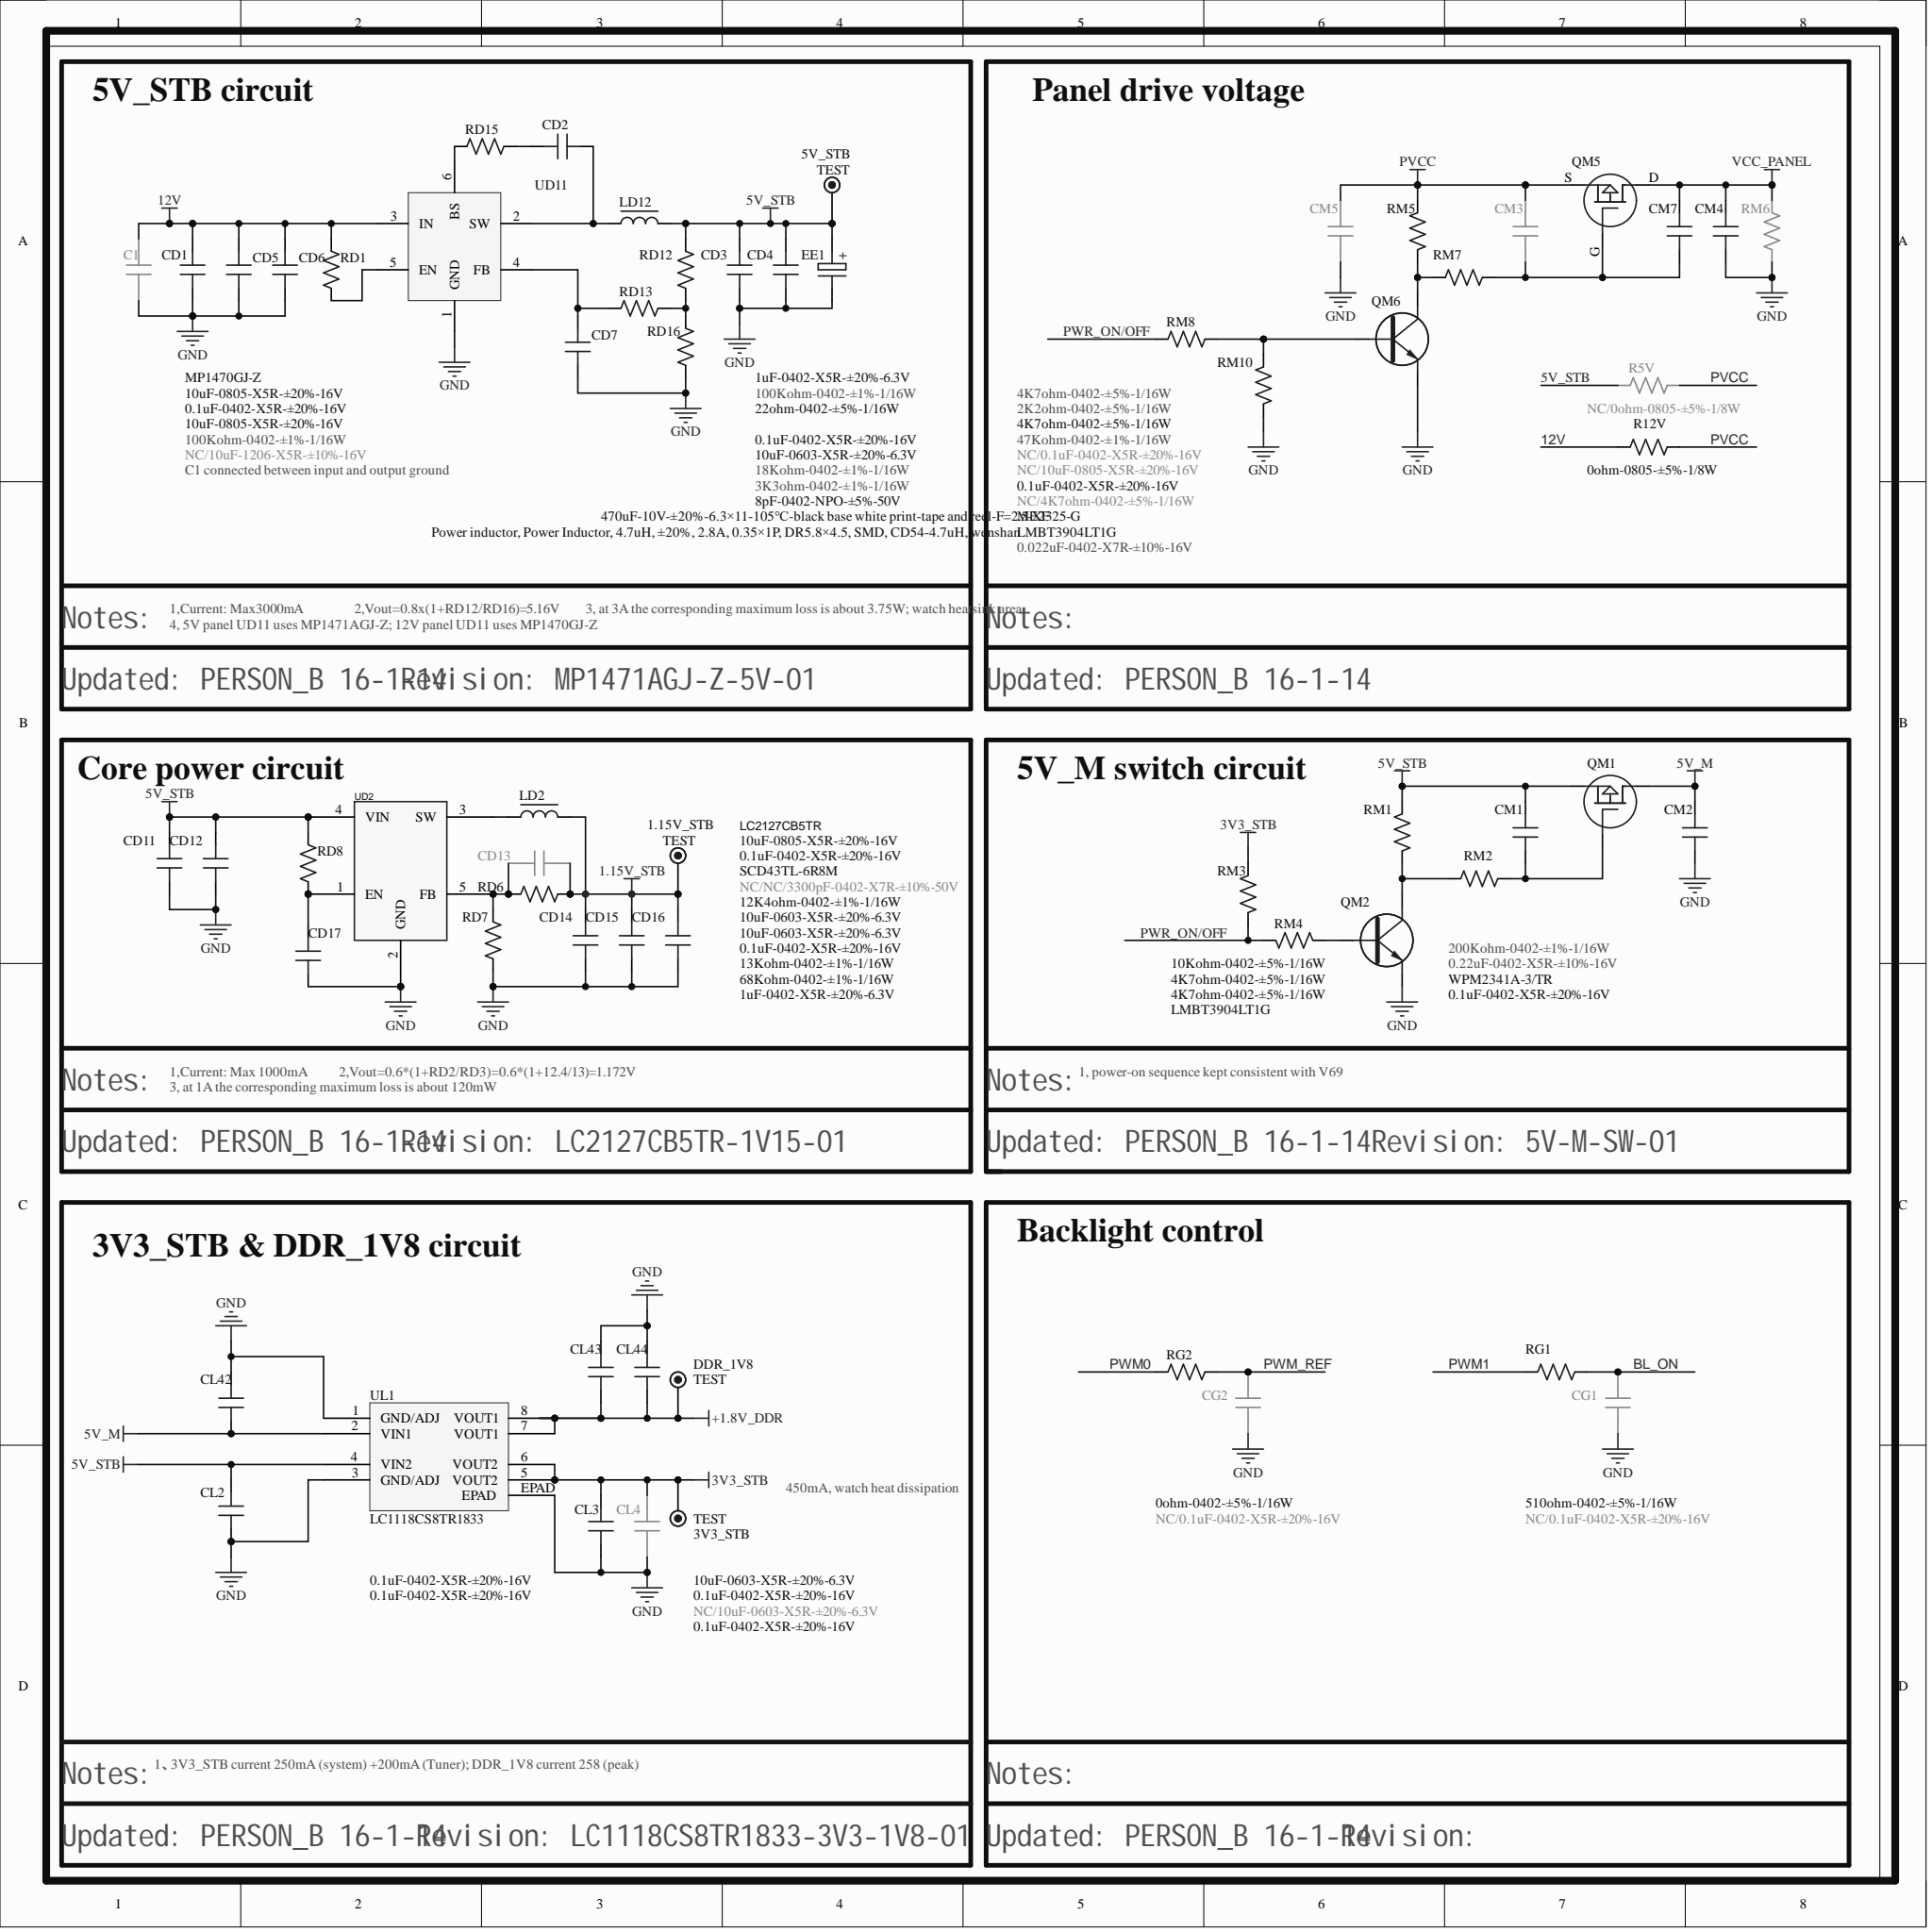Circuit board | Altium Designer | 709 parts | 378 nets | one sheet of the schematic
Parts on this sheet (reference | value | footprint):
1.15V_STB | TEST | TP
3V3_STB | TEST | TP
5V_STB | TEST | TP
BL_ON | TEST | TP_BL
C1 | NC/10uF-1206-X5R-±10%-16V | C1206
CD1 | 10uF-0805-X5R-±20%-16V | C0805
CD2 | 1uF-0402-X5R-±20%-6.3V | C0402
CD3 | 0.1uF-0402-X5R-±20%-16V | C0402
CD4 | 10uF-0603-X5R-±20%-6.3V | C0603
CD5 | 10uF-0805-X5R-±20%-16V | C0805
CD6 | 0.1uF-0402-X5R-±20%-16V | C0402
CD7 | 8pF-0402-NPO-±5%-50V | C0402
CD11 | 10uF-0805-X5R-±20%-16V | C0805
CD12 | 0.1uF-0402-X5R-±20%-16V | C0402
CD13 | NC/NC/3300pF-0402-X7R-±10%-50V | C0402
CD14 | 10uF-0603-X5R-±20%-6.3V | C0603
CD15 | 10uF-0603-X5R-±20%-6.3V | C0603
CD16 | 0.1uF-0402-X5R-±20%-16V | C0402
CD17 | 1uF-0402-X5R-±20%-6.3V | C0402
CG1 | NC/0.1uF-0402-X5R-±20%-16V | C0402
CG2 | NC/0.1uF-0402-X5R-±20%-16V | C0402
CL2 | 0.1uF-0402-X5R-±20%-16V | C0402
CL3 | 0.1uF-0402-X5R-±20%-16V | C0402
CL4 | NC/10uF-0603-X5R-±20%-6.3V | C0603
CL42 | 0.1uF-0402-X5R-±20%-16V | C0402
CL43 | 0.1uF-0402-X5R-±20%-16V | C0402
CL44 | 10uF-0603-X5R-±20%-6.3V | C0603
CM1 | 0.22uF-0402-X5R-±10%-16V | C0402
CM2 | 0.1uF-0402-X5R-±20%-16V | C0402
CM3 | NC/0.1uF-0402-X5R-±20%-16V | C0402
CM4 | 0.1uF-0402-X5R-±20%-16V | C0402
CM5 | NC/10uF-0805-X5R-±20%-16V | C0805
CM7 | 0.022uF-0402-X7R-±10%-16V | C0402
DDR_1V8 | TEST | TP
EE1 | 470uF-10V-±20%-6.3×11-105℃-black base white print-tape and reel-F=2.5-XF | EC(6.3*11)-V-2.5
LD2 | SCD43TL-6R8M | L(4.5*3.5)-S
LD12 | Power inductor, Power Inductor, 4.7uH, ±20%, 2.8A, 0.35×1P, DR5.8×4.5, SMD, CD54-4.7uH, wenshan | L(5.8*4.5)-S
PWM_REF | TEST | TP_BL
QM1 | WPM2341A-3/TR | SOT-23-1
QM2 | LMBT3904LT1G | SOT-23
QM5 | ME2325-G | SOT-23-1
QM6 | LMBT3904LT1G | SOT-23
R5V | NC/0ohm-0805-±5%-1/8W | R0805
R12V | 0ohm-0805-±5%-1/8W | R0805
RD1 | 100Kohm-0402-±1%-1/16W | R0402
RD6 | 12K4ohm-0402-±1%-1/16W | R0402
RD7 | 13Kohm-0402-±1%-1/16W | R0402
RD8 | 68Kohm-0402-±1%-1/16W | R0402
RD12 | 18Kohm-0402-±1%-1/16W | R0402
RD13 | 100Kohm-0402-±1%-1/16W | R0402
RD15 | 22ohm-0402-±5%-1/16W | R0402
RD16 | 3K3ohm-0402-±1%-1/16W | R0402
RG1 | 510ohm-0402-±5%-1/16W | R0402
RG2 | 0ohm-0402-±5%-1/16W | R0402
RM1 | 4K7ohm-0402-±5%-1/16W | R0402
RM2 | 200Kohm-0402-±1%-1/16W | R0402
RM3 | 10Kohm-0402-±5%-1/16W | R0402
RM4 | 4K7ohm-0402-±5%-1/16W | R0402
RM5 | 4K7ohm-0402-±5%-1/16W | R0402
RM6 | NC/4K7ohm-0402-±5%-1/16W | R0402
RM7 | 47Kohm-0402-±1%-1/16W | R0402
RM8 | 4K7ohm-0402-±5%-1/16W | R0402
RM10 | 2K2ohm-0402-±5%-1/16W | R0402
UD2 | LC2127CB5TR | SOT-23-5
UD11 | MP1470GJ-Z | SOT-23-6
UL1 | LC1118CS8TR1833 | SOP8/1.27-3
Nets of these parts (net: part-pin ...):
VCC_PANEL: CM4-1 CM7-1 QM5-D RM6-1
PWR_ON/OFF: RM3-2 RM4-2 RM8-1
PWM_REF: CG2-1 PWM_REF-1 RG2-2
PWM1: RG1-2
PWM0: RG2-1
PVCC: CM3-2 CM5-2 QM5-S R5V-2 R12V-2 RM5-2
NetRD15_1: RD15-1 UD11-6
NetRD12_1: RD12-1 RD13-1 RD16-2
NetRD1_2: RD1-2 UD11-5
NetQM6_C: QM6-C RM5-1 RM7-1
NetQM6_B: QM6-B RM8-2 RM10-1
NetQM2_C: QM2-C RM1-1 RM2-1
NetQM2_B: QM2-B RM4-1
NetLD2_1: LD2-1 UD2-3
NetCM3_1: CM3-1 CM7-2 QM5-G RM7-2
NetCM1_2: CM1-2 QM1-G RM2-2
NetCD17_2: CD17-2 RD8-2 UD2-1
NetCD13_2: CD13-2 RD6-1 RD7-2 UD2-5
NetCD7_1: CD7-1 RD13-2 UD11-4
NetCD2_2: CD2-2 RD15-2
NetCD2_1: CD2-1 LD12-1 UD11-2
GND: C1-1 CD1-2 CD3-2 CD4-1 CD5-2 CD6-2 CD7-2 CD11-1 CD12-2 CD14-1 CD15-1 CD16-1 CD17-1 CG1-2 CG2-2 CL2-1 CL3-2 CL4-2 CL42-2 CL43-1 CL44-2 CM2-2 CM4-2 CM5-1 EE1-2 QM2-E QM6-E RD7-1 RD16-1 RM6-2 RM10-2 UD2-2 UD11-1 UL1-1 UL1-3 UL1-EPAD
BL_ON: BL_ON-1 CG1-1 RG1-1
+1.8V_DDR: CL43-2 CL44-1 DDR_1V8-1 UL1-7 UL1-8
12V: C1-2 CD1-1 CD5-1 CD6-1 R12V-1 RD1-1 UD11-3
5V_STB: 5V_STB-1 CD3-1 CD4-2 CD11-2 CD12-1 CL2-2 CM1-1 EE1-1 LD12-2 QM1-S R5V-1 RD8-1 RD12-2 RM1-2 UD2-4 UL1-4
5V_M: CL42-1 CM2-1 QM1-D UL1-2
3V3_STB: 3V3_STB-1 CL3-1 CL4-1 RM3-1 UL1-5 UL1-6
1.15V_STB: 1.15V_STB-1 CD13-1 CD14-2 CD15-2 CD16-2 LD2-2 RD6-2